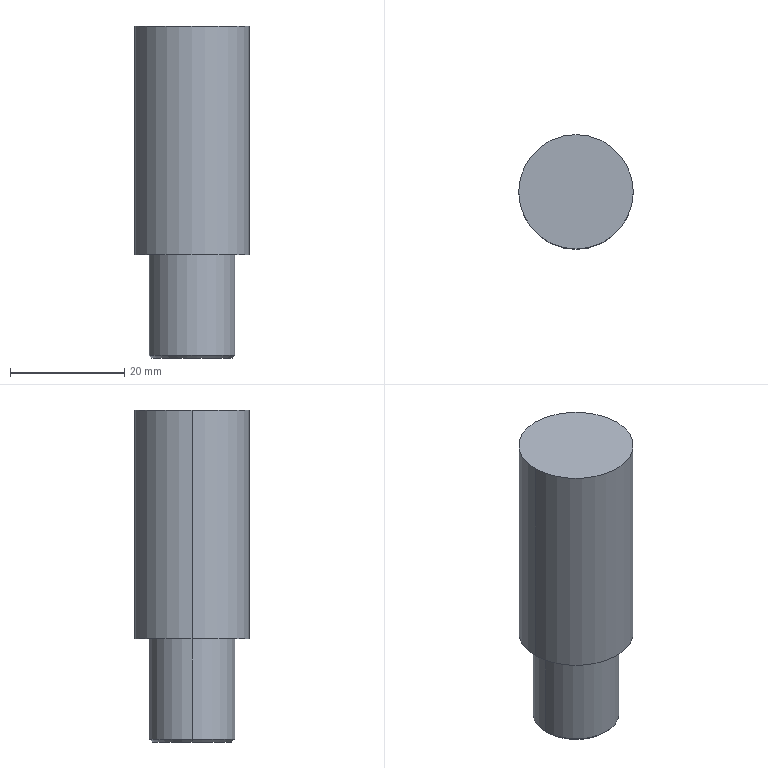Part | SolidWorks | features BaseBody 1 | 1 solid | 13 faces | box 20 x 20 x 58 mm | volume 14909 mm3 | cylinder 6 | cone 4 | plane 3 | commonest cylinder face diameters 6.8 x2 15 x2 20 x2
STEP:
#1=CARTESIAN_POINT('',(-7.,0.,-18.));
#2=VERTEX_POINT('',#1);
#3=CARTESIAN_POINT('',(-7.5,0.,-17.5));
#4=VERTEX_POINT('',#3);
#5=CARTESIAN_POINT('',(-7.,0.,-18.));
#6=DIRECTION('',(-0.7071,0.,0.7071));
#7=VECTOR('',#6,1000.);
#8=LINE('',#5,#7);
#9=EDGE_CURVE('',#2,#4,#8,.T.);
#10=ORIENTED_EDGE('',*,*,#9,.F.);
#11=CARTESIAN_POINT('',(7.,0.,-18.));
#12=VERTEX_POINT('',#11);
#13=CARTESIAN_POINT('',(0.,0.,-18.));
#14=DIRECTION('',(0.,0.,-1.));
#15=DIRECTION('',(-1.,0.,0.));
#16=AXIS2_PLACEMENT_3D('',#13,#14,#15);
#17=CIRCLE('',#16,7.);
#18=EDGE_CURVE('',#12,#2,#17,.T.);
#19=ORIENTED_EDGE('',*,*,#18,.F.);
#20=CARTESIAN_POINT('',(7.5,0.,-17.5));
#21=VERTEX_POINT('',#20);
#22=CARTESIAN_POINT('',(7.,0.,-18.));
#23=DIRECTION('',(0.7071,0.,0.7071));
#24=VECTOR('',#23,1000.);
#25=LINE('',#22,#24);
#26=EDGE_CURVE('',#12,#21,#25,.T.);
#27=ORIENTED_EDGE('',*,*,#26,.T.);
#28=CARTESIAN_POINT('',(0.,0.,-17.5));
#29=DIRECTION('',(0.,0.,1.));
#30=DIRECTION('',(-1.,0.,0.));
#31=AXIS2_PLACEMENT_3D('',#28,#29,#30);
#32=CIRCLE('',#31,7.5);
#33=EDGE_CURVE('',#4,#21,#32,.T.);
#34=ORIENTED_EDGE('',*,*,#33,.F.);
#35=EDGE_LOOP('',(#10,#19,#27,#34));
#36=FACE_OUTER_BOUND('',#35,.T.);
#37=CARTESIAN_POINT('',(0.,0.,-18.));
#38=DIRECTION('',(0.,0.,1.));
#39=DIRECTION('',(1.,0.,0.));
#40=AXIS2_PLACEMENT_3D('',#37,#38,#39);
#41=CONICAL_SURFACE('',#40,7.,0.7854);
#42=ADVANCED_FACE('',(#36),#41,.T.);
#43=CARTESIAN_POINT('',(3.4,0.,4.25));
#44=VERTEX_POINT('',#43);
#45=CARTESIAN_POINT('',(3.4,0.,-18.));
#46=VERTEX_POINT('',#45);
#47=CARTESIAN_POINT('',(3.4,0.,-18.));
#48=DIRECTION('',(0.,0.,-1.));
#49=VECTOR('',#48,1000.);
#50=LINE('',#47,#49);
#51=EDGE_CURVE('',#44,#46,#50,.T.);
#52=ORIENTED_EDGE('',*,*,#51,.F.);
#53=CARTESIAN_POINT('',(-3.4,0.,4.25));
#54=VERTEX_POINT('',#53);
#55=CARTESIAN_POINT('',(0.,0.,4.25));
#56=DIRECTION('',(0.,0.,-1.));
#57=DIRECTION('',(-1.,0.,0.));
#58=AXIS2_PLACEMENT_3D('',#55,#56,#57);
#59=CIRCLE('',#58,3.4);
#60=EDGE_CURVE('',#54,#44,#59,.T.);
#61=ORIENTED_EDGE('',*,*,#60,.F.);
#62=CARTESIAN_POINT('',(-3.4,0.,-18.));
#63=VERTEX_POINT('',#62);
#64=CARTESIAN_POINT('',(-3.4,0.,-18.));
#65=DIRECTION('',(0.,0.,-1.));
#66=VECTOR('',#65,1000.);
#67=LINE('',#64,#66);
#68=EDGE_CURVE('',#54,#63,#67,.T.);
#69=ORIENTED_EDGE('',*,*,#68,.T.);
#70=CARTESIAN_POINT('',(0.,0.,-18.));
#71=DIRECTION('',(0.,0.,-1.));
#72=DIRECTION('',(-1.,0.,0.));
#73=AXIS2_PLACEMENT_3D('',#70,#71,#72);
#74=CIRCLE('',#73,3.4);
#75=EDGE_CURVE('',#63,#46,#74,.T.);
#76=ORIENTED_EDGE('',*,*,#75,.T.);
#77=EDGE_LOOP('',(#52,#61,#69,#76));
#78=FACE_OUTER_BOUND('',#77,.T.);
#79=CARTESIAN_POINT('',(0.,0.,-18.));
#80=DIRECTION('',(0.,0.,-1.));
#81=DIRECTION('',(-1.,0.,0.));
#82=AXIS2_PLACEMENT_3D('',#79,#80,#81);
#83=CYLINDRICAL_SURFACE('',#82,3.4);
#84=ADVANCED_FACE('',(#78),#83,.F.);
#85=CARTESIAN_POINT('',(0.,0.,6.293));
#86=VERTEX_POINT('',#85);
#87=CARTESIAN_POINT('',(3.4,0.,4.25));
#88=DIRECTION('',(0.8572,0.,-0.515));
#89=VECTOR('',#88,1000.);
#90=LINE('',#87,#89);
#91=EDGE_CURVE('',#86,#44,#90,.T.);
#92=ORIENTED_EDGE('',*,*,#91,.F.);
#93=CARTESIAN_POINT('',(-3.4,0.,4.25));
#94=DIRECTION('',(-0.8572,0.,-0.515));
#95=VECTOR('',#94,1000.);
#96=LINE('',#93,#95);
#97=EDGE_CURVE('',#86,#54,#96,.T.);
#98=ORIENTED_EDGE('',*,*,#97,.T.);
#99=ORIENTED_EDGE('',*,*,#60,.T.);
#100=EDGE_LOOP('',(#92,#98,#99));
#101=FACE_OUTER_BOUND('',#100,.T.);
#102=CARTESIAN_POINT('',(0.,0.,4.25));
#103=DIRECTION('',(0.,0.,-1.));
#104=DIRECTION('',(-1.,0.,0.));
#105=AXIS2_PLACEMENT_3D('',#102,#103,#104);
#106=CONICAL_SURFACE('',#105,3.4,1.03);
#107=ADVANCED_FACE('',(#101),#106,.F.);
#108=ORIENTED_EDGE('',*,*,#75,.F.);
#109=CARTESIAN_POINT('',(0.,0.,-18.));
#110=DIRECTION('',(0.,0.,-1.));
#111=DIRECTION('',(-1.,0.,0.));
#112=AXIS2_PLACEMENT_3D('',#109,#110,#111);
#113=CIRCLE('',#112,3.4);
#114=EDGE_CURVE('',#46,#63,#113,.T.);
#115=ORIENTED_EDGE('',*,*,#114,.F.);
#116=EDGE_LOOP('',(#108,#115));
#117=FACE_BOUND('',#116,.T.);
#118=ORIENTED_EDGE('',*,*,#18,.T.);
#119=CARTESIAN_POINT('',(0.,0.,-18.));
#120=DIRECTION('',(0.,0.,-1.));
#121=DIRECTION('',(-1.,0.,0.));
#122=AXIS2_PLACEMENT_3D('',#119,#120,#121);
#123=CIRCLE('',#122,7.);
#124=EDGE_CURVE('',#2,#12,#123,.T.);
#125=ORIENTED_EDGE('',*,*,#124,.T.);
#126=EDGE_LOOP('',(#118,#125));
#127=FACE_OUTER_BOUND('',#126,.T.);
#128=CARTESIAN_POINT('',(0.,0.,-18.));
#129=DIRECTION('',(0.,0.,-1.));
#130=DIRECTION('',(0.,-1.,0.));
#131=AXIS2_PLACEMENT_3D('',#128,#129,#130);
#132=PLANE('',#131);
#133=ADVANCED_FACE('',(#117,#127),#132,.T.);
#134=CARTESIAN_POINT('',(-7.5,0.,0.));
#135=VERTEX_POINT('',#134);
#136=CARTESIAN_POINT('',(-7.5,0.,-18.));
#137=DIRECTION('',(0.,0.,1.));
#138=VECTOR('',#137,1000.);
#139=LINE('',#136,#138);
#140=EDGE_CURVE('',#4,#135,#139,.T.);
#141=ORIENTED_EDGE('',*,*,#140,.F.);
#142=ORIENTED_EDGE('',*,*,#33,.T.);
#143=CARTESIAN_POINT('',(7.5,0.,0.));
#144=VERTEX_POINT('',#143);
#145=CARTESIAN_POINT('',(7.5,0.,-18.));
#146=DIRECTION('',(0.,0.,1.));
#147=VECTOR('',#146,1000.);
#148=LINE('',#145,#147);
#149=EDGE_CURVE('',#21,#144,#148,.T.);
#150=ORIENTED_EDGE('',*,*,#149,.T.);
#151=CARTESIAN_POINT('',(0.,0.,0.));
#152=DIRECTION('',(0.,0.,-1.));
#153=DIRECTION('',(-1.,0.,0.));
#154=AXIS2_PLACEMENT_3D('',#151,#152,#153);
#155=CIRCLE('',#154,7.5);
#156=EDGE_CURVE('',#144,#135,#155,.T.);
#157=ORIENTED_EDGE('',*,*,#156,.T.);
#158=EDGE_LOOP('',(#141,#142,#150,#157));
#159=FACE_OUTER_BOUND('',#158,.T.);
#160=CARTESIAN_POINT('',(0.,0.,-18.));
#161=DIRECTION('',(0.,0.,1.));
#162=DIRECTION('',(1.,0.,0.));
#163=AXIS2_PLACEMENT_3D('',#160,#161,#162);
#164=CYLINDRICAL_SURFACE('',#163,7.5);
#165=ADVANCED_FACE('',(#159),#164,.T.);
#166=ORIENTED_EDGE('',*,*,#156,.F.);
#167=CARTESIAN_POINT('',(0.,0.,0.));
#168=DIRECTION('',(0.,0.,-1.));
#169=DIRECTION('',(-1.,0.,0.));
#170=AXIS2_PLACEMENT_3D('',#167,#168,#169);
#171=CIRCLE('',#170,7.5);
#172=EDGE_CURVE('',#135,#144,#171,.T.);
#173=ORIENTED_EDGE('',*,*,#172,.F.);
#174=EDGE_LOOP('',(#166,#173));
#175=FACE_BOUND('',#174,.T.);
#176=CARTESIAN_POINT('',(-10.,0.,0.));
#177=VERTEX_POINT('',#176);
#178=CARTESIAN_POINT('',(10.,0.,0.));
#179=VERTEX_POINT('',#178);
#180=CARTESIAN_POINT('',(0.,0.,0.));
#181=DIRECTION('',(0.,0.,1.));
#182=DIRECTION('',(1.,0.,0.));
#183=AXIS2_PLACEMENT_3D('',#180,#181,#182);
#184=CIRCLE('',#183,10.);
#185=EDGE_CURVE('',#177,#179,#184,.T.);
#186=ORIENTED_EDGE('',*,*,#185,.F.);
#187=CARTESIAN_POINT('',(0.,0.,0.));
#188=DIRECTION('',(0.,0.,1.));
#189=DIRECTION('',(1.,0.,0.));
#190=AXIS2_PLACEMENT_3D('',#187,#188,#189);
#191=CIRCLE('',#190,10.);
#192=EDGE_CURVE('',#179,#177,#191,.T.);
#193=ORIENTED_EDGE('',*,*,#192,.F.);
#194=EDGE_LOOP('',(#186,#193));
#195=FACE_OUTER_BOUND('',#194,.T.);
#196=CARTESIAN_POINT('',(0.,0.,0.));
#197=DIRECTION('',(0.,0.,1.));
#198=DIRECTION('',(1.,0.,0.));
#199=AXIS2_PLACEMENT_3D('',#196,#197,#198);
#200=PLANE('',#199);
#201=ADVANCED_FACE('',(#175,#195),#200,.F.);
#202=CARTESIAN_POINT('',(-10.,0.,40.));
#203=VERTEX_POINT('',#202);
#204=CARTESIAN_POINT('',(10.,0.,40.));
#205=VERTEX_POINT('',#204);
#206=CARTESIAN_POINT('',(0.,0.,40.));
#207=DIRECTION('',(0.,0.,1.));
#208=DIRECTION('',(1.,0.,0.));
#209=AXIS2_PLACEMENT_3D('',#206,#207,#208);
#210=CIRCLE('',#209,10.);
#211=EDGE_CURVE('',#203,#205,#210,.T.);
#212=ORIENTED_EDGE('',*,*,#211,.T.);
#213=CARTESIAN_POINT('',(0.,0.,40.));
#214=DIRECTION('',(0.,0.,1.));
#215=DIRECTION('',(1.,0.,0.));
#216=AXIS2_PLACEMENT_3D('',#213,#214,#215);
#217=CIRCLE('',#216,10.);
#218=EDGE_CURVE('',#205,#203,#217,.T.);
#219=ORIENTED_EDGE('',*,*,#218,.T.);
#220=EDGE_LOOP('',(#212,#219));
#221=FACE_OUTER_BOUND('',#220,.T.);
#222=CARTESIAN_POINT('',(0.,0.,40.));
#223=DIRECTION('',(0.,0.,1.));
#224=DIRECTION('',(1.,0.,0.));
#225=AXIS2_PLACEMENT_3D('',#222,#223,#224);
#226=PLANE('',#225);
#227=ADVANCED_FACE('',(#221),#226,.T.);
#228=CARTESIAN_POINT('',(10.,0.,40.));
#229=DIRECTION('',(0.,0.,-1.));
#230=VECTOR('',#229,1000.);
#231=LINE('',#228,#230);
#232=EDGE_CURVE('',#205,#179,#231,.T.);
#233=ORIENTED_EDGE('',*,*,#232,.F.);
#234=ORIENTED_EDGE('',*,*,#211,.F.);
#235=CARTESIAN_POINT('',(-10.,0.,40.));
#236=DIRECTION('',(0.,0.,-1.));
#237=VECTOR('',#236,1000.);
#238=LINE('',#235,#237);
#239=EDGE_CURVE('',#203,#177,#238,.T.);
#240=ORIENTED_EDGE('',*,*,#239,.T.);
#241=ORIENTED_EDGE('',*,*,#185,.T.);
#242=EDGE_LOOP('',(#233,#234,#240,#241));
#243=FACE_OUTER_BOUND('',#242,.T.);
#244=CARTESIAN_POINT('',(0.,0.,40.));
#245=DIRECTION('',(0.,0.,-1.));
#246=DIRECTION('',(-1.,0.,0.));
#247=AXIS2_PLACEMENT_3D('',#244,#245,#246);
#248=CYLINDRICAL_SURFACE('',#247,10.);
#249=ADVANCED_FACE('',(#243),#248,.T.);
#250=ORIENTED_EDGE('',*,*,#218,.F.);
#251=ORIENTED_EDGE('',*,*,#232,.T.);
#252=ORIENTED_EDGE('',*,*,#192,.T.);
#253=ORIENTED_EDGE('',*,*,#239,.F.);
#254=EDGE_LOOP('',(#250,#251,#252,#253));
#255=FACE_OUTER_BOUND('',#254,.T.);
#256=CARTESIAN_POINT('',(0.,0.,40.));
#257=DIRECTION('',(0.,0.,-1.));
#258=DIRECTION('',(-1.,0.,0.));
#259=AXIS2_PLACEMENT_3D('',#256,#257,#258);
#260=CYLINDRICAL_SURFACE('',#259,10.);
#261=ADVANCED_FACE('',(#255),#260,.T.);
#262=CARTESIAN_POINT('',(0.,0.,-17.5));
#263=DIRECTION('',(0.,0.,1.));
#264=DIRECTION('',(-1.,0.,0.));
#265=AXIS2_PLACEMENT_3D('',#262,#263,#264);
#266=CIRCLE('',#265,7.5);
#267=EDGE_CURVE('',#21,#4,#266,.T.);
#268=ORIENTED_EDGE('',*,*,#267,.T.);
#269=ORIENTED_EDGE('',*,*,#140,.T.);
#270=ORIENTED_EDGE('',*,*,#172,.T.);
#271=ORIENTED_EDGE('',*,*,#149,.F.);
#272=EDGE_LOOP('',(#268,#269,#270,#271));
#273=FACE_OUTER_BOUND('',#272,.T.);
#274=CARTESIAN_POINT('',(0.,0.,-18.));
#275=DIRECTION('',(0.,0.,1.));
#276=DIRECTION('',(1.,0.,0.));
#277=AXIS2_PLACEMENT_3D('',#274,#275,#276);
#278=CYLINDRICAL_SURFACE('',#277,7.5);
#279=ADVANCED_FACE('',(#273),#278,.T.);
#280=ORIENTED_EDGE('',*,*,#97,.F.);
#281=ORIENTED_EDGE('',*,*,#91,.T.);
#282=CARTESIAN_POINT('',(0.,0.,4.25));
#283=DIRECTION('',(0.,0.,-1.));
#284=DIRECTION('',(-1.,0.,0.));
#285=AXIS2_PLACEMENT_3D('',#282,#283,#284);
#286=CIRCLE('',#285,3.4);
#287=EDGE_CURVE('',#44,#54,#286,.T.);
#288=ORIENTED_EDGE('',*,*,#287,.T.);
#289=EDGE_LOOP('',(#280,#281,#288));
#290=FACE_OUTER_BOUND('',#289,.T.);
#291=CARTESIAN_POINT('',(0.,0.,4.25));
#292=DIRECTION('',(0.,0.,-1.));
#293=DIRECTION('',(-1.,0.,0.));
#294=AXIS2_PLACEMENT_3D('',#291,#292,#293);
#295=CONICAL_SURFACE('',#294,3.4,1.03);
#296=ADVANCED_FACE('',(#290),#295,.F.);
#297=ORIENTED_EDGE('',*,*,#287,.F.);
#298=ORIENTED_EDGE('',*,*,#51,.T.);
#299=ORIENTED_EDGE('',*,*,#114,.T.);
#300=ORIENTED_EDGE('',*,*,#68,.F.);
#301=EDGE_LOOP('',(#297,#298,#299,#300));
#302=FACE_OUTER_BOUND('',#301,.T.);
#303=CARTESIAN_POINT('',(0.,0.,-18.));
#304=DIRECTION('',(0.,0.,-1.));
#305=DIRECTION('',(-1.,0.,0.));
#306=AXIS2_PLACEMENT_3D('',#303,#304,#305);
#307=CYLINDRICAL_SURFACE('',#306,3.4);
#308=ADVANCED_FACE('',(#302),#307,.F.);
#309=ORIENTED_EDGE('',*,*,#124,.F.);
#310=ORIENTED_EDGE('',*,*,#9,.T.);
#311=ORIENTED_EDGE('',*,*,#267,.F.);
#312=ORIENTED_EDGE('',*,*,#26,.F.);
#313=EDGE_LOOP('',(#309,#310,#311,#312));
#314=FACE_OUTER_BOUND('',#313,.T.);
#315=CARTESIAN_POINT('',(0.,0.,-18.));
#316=DIRECTION('',(0.,0.,1.));
#317=DIRECTION('',(1.,0.,0.));
#318=AXIS2_PLACEMENT_3D('',#315,#316,#317);
#319=CONICAL_SURFACE('',#318,7.,0.7854);
#320=ADVANCED_FACE('',(#314),#319,.T.);
#321=CLOSED_SHELL('',(#42,#84,#107,#133,#165,#201,#227,#249,#261,#279,#296,#308,#320));
#322=MANIFOLD_SOLID_BREP('',#321);
#323=CARTESIAN_POINT('',(0.,0.,0.));
#324=DIRECTION('',(0.,0.,1.));
#325=DIRECTION('',(1.,0.,0.));
#326=AXIS2_PLACEMENT_3D('',#323,#324,#325);
#327=(LENGTH_UNIT()NAMED_UNIT(*)SI_UNIT(.MILLI.,.METRE.));
#328=UNCERTAINTY_MEASURE_WITH_UNIT(LENGTH_MEASURE(0.00001),#327,'','');
#329=(NAMED_UNIT(*)PLANE_ANGLE_UNIT()SI_UNIT($,.RADIAN.));
#330=(NAMED_UNIT(*)SI_UNIT($,.STERADIAN.)SOLID_ANGLE_UNIT());
#331=(GEOMETRIC_REPRESENTATION_CONTEXT(3)GLOBAL_UNCERTAINTY_ASSIGNED_CONTEXT((#328))GLOBAL_UNIT_ASSIGNED_CONTEXT((#327,#329,#330))REPRESENTATION_CONTEXT('',''));
#332=ADVANCED_BREP_SHAPE_REPRESENTATION('',(#322,#326),#331);